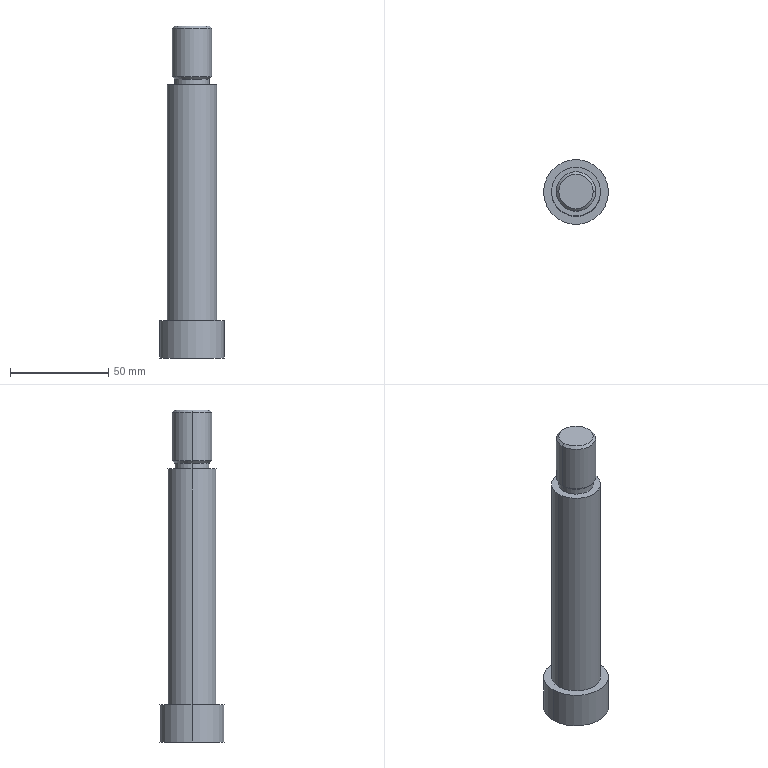Part | Creo | 1 solid | 23 faces | box 33 x 33 x 169 mm | volume 81512 mm3 | plane 11 | cylinder 8 | cone 4 | commonest cylinder face diameters 17.5 x2 20 x2 25 x2 33 x2
STEP:
#1=CARTESIAN_POINT('',(-191.5,290.,11.5));
#2=VERTEX_POINT('',#1);
#3=CARTESIAN_POINT('',(-158.5,290.,11.5));
#4=VERTEX_POINT('',#3);
#5=CARTESIAN_POINT('',(-175.,290.,11.5));
#6=DIRECTION('',(0.,0.,-1.));
#7=DIRECTION('',(-1.,0.,0.));
#8=AXIS2_PLACEMENT_3D('',#5,#6,#7);
#9=CIRCLE('',#8,16.5);
#10=EDGE_CURVE('',#2,#4,#9,.T.);
#11=ORIENTED_EDGE('',*,*,#10,.F.);
#12=CARTESIAN_POINT('',(-175.,290.,11.5));
#13=DIRECTION('',(0.,0.,-1.));
#14=DIRECTION('',(1.,0.,0.));
#15=AXIS2_PLACEMENT_3D('',#12,#13,#14);
#16=CIRCLE('',#15,16.5);
#17=EDGE_CURVE('',#4,#2,#16,.T.);
#18=ORIENTED_EDGE('',*,*,#17,.F.);
#19=EDGE_LOOP('',(#11,#18));
#20=FACE_OUTER_BOUND('',#19,.F.);
#21=CARTESIAN_POINT('',(-166.5,294.907,11.5));
#22=VERTEX_POINT('',#21);
#23=CARTESIAN_POINT('',(-175.,299.815,11.5));
#24=VERTEX_POINT('',#23);
#25=CARTESIAN_POINT('',(-166.5,294.907,11.5));
#26=DIRECTION('',(-0.866,0.5,0.));
#27=VECTOR('',#26,9.815);
#28=LINE('',#25,#27);
#29=EDGE_CURVE('',#22,#24,#28,.T.);
#30=ORIENTED_EDGE('',*,*,#29,.F.);
#31=CARTESIAN_POINT('',(-166.5,285.093,11.5));
#32=VERTEX_POINT('',#31);
#33=CARTESIAN_POINT('',(-166.5,285.093,11.5));
#34=DIRECTION('',(0.,1.,0.));
#35=VECTOR('',#34,9.815);
#36=LINE('',#33,#35);
#37=EDGE_CURVE('',#32,#22,#36,.T.);
#38=ORIENTED_EDGE('',*,*,#37,.F.);
#39=CARTESIAN_POINT('',(-175.,280.185,11.5));
#40=VERTEX_POINT('',#39);
#41=CARTESIAN_POINT('',(-175.,280.185,11.5));
#42=DIRECTION('',(0.866,0.5,0.));
#43=VECTOR('',#42,9.815);
#44=LINE('',#41,#43);
#45=EDGE_CURVE('',#40,#32,#44,.T.);
#46=ORIENTED_EDGE('',*,*,#45,.F.);
#47=CARTESIAN_POINT('',(-183.5,285.093,11.5));
#48=VERTEX_POINT('',#47);
#49=CARTESIAN_POINT('',(-183.5,285.093,11.5));
#50=DIRECTION('',(0.866,-0.5,0.));
#51=VECTOR('',#50,9.815);
#52=LINE('',#49,#51);
#53=EDGE_CURVE('',#48,#40,#52,.T.);
#54=ORIENTED_EDGE('',*,*,#53,.F.);
#55=CARTESIAN_POINT('',(-183.5,294.907,11.5));
#56=VERTEX_POINT('',#55);
#57=CARTESIAN_POINT('',(-183.5,285.093,11.5));
#58=DIRECTION('',(0.,1.,0.));
#59=VECTOR('',#58,9.815);
#60=LINE('',#57,#59);
#61=EDGE_CURVE('',#48,#56,#60,.T.);
#62=ORIENTED_EDGE('',*,*,#61,.T.);
#63=CARTESIAN_POINT('',(-175.,299.815,11.5));
#64=DIRECTION('',(-0.866,-0.5,0.));
#65=VECTOR('',#64,9.815);
#66=LINE('',#63,#65);
#67=EDGE_CURVE('',#24,#56,#66,.T.);
#68=ORIENTED_EDGE('',*,*,#67,.F.);
#69=EDGE_LOOP('',(#30,#38,#46,#54,#62,#68));
#70=FACE_BOUND('',#69,.F.);
#71=CARTESIAN_POINT('',(-175.,290.,11.5));
#72=DIRECTION('',(0.,0.,-1.));
#73=DIRECTION('',(-1.,0.,0.));
#74=AXIS2_PLACEMENT_3D('',#71,#72,#73);
#75=PLANE('',#74);
#76=ADVANCED_FACE('',(#20,#70),#75,.T.);
#77=ORIENTED_EDGE('',*,*,#29,.T.);
#78=CARTESIAN_POINT('',(-175.,299.815,22.5));
#79=VERTEX_POINT('',#78);
#80=CARTESIAN_POINT('',(-175.,299.815,11.5));
#81=DIRECTION('',(0.,0.,1.));
#82=VECTOR('',#81,11.);
#83=LINE('',#80,#82);
#84=EDGE_CURVE('',#24,#79,#83,.T.);
#85=ORIENTED_EDGE('',*,*,#84,.T.);
#86=CARTESIAN_POINT('',(-166.5,294.907,22.5));
#87=VERTEX_POINT('',#86);
#88=CARTESIAN_POINT('',(-175.,299.815,22.5));
#89=DIRECTION('',(0.866,-0.5,0.));
#90=VECTOR('',#89,9.815);
#91=LINE('',#88,#90);
#92=EDGE_CURVE('',#79,#87,#91,.T.);
#93=ORIENTED_EDGE('',*,*,#92,.T.);
#94=CARTESIAN_POINT('',(-166.5,294.907,22.5));
#95=DIRECTION('',(0.,0.,-1.));
#96=VECTOR('',#95,11.);
#97=LINE('',#94,#96);
#98=EDGE_CURVE('',#87,#22,#97,.T.);
#99=ORIENTED_EDGE('',*,*,#98,.T.);
#100=EDGE_LOOP('',(#77,#85,#93,#99));
#101=FACE_OUTER_BOUND('',#100,.F.);
#102=CARTESIAN_POINT('',(-170.75,297.361,30.5));
#103=DIRECTION('',(0.5,0.866,0.));
#104=DIRECTION('',(-0.866,0.5,0.));
#105=AXIS2_PLACEMENT_3D('',#102,#103,#104);
#106=PLANE('',#105);
#107=ADVANCED_FACE('',(#101),#106,.F.);
#108=ORIENTED_EDGE('',*,*,#67,.T.);
#109=CARTESIAN_POINT('',(-183.5,294.907,22.5));
#110=VERTEX_POINT('',#109);
#111=CARTESIAN_POINT('',(-183.5,294.907,22.5));
#112=DIRECTION('',(0.,0.,-1.));
#113=VECTOR('',#112,11.);
#114=LINE('',#111,#113);
#115=EDGE_CURVE('',#110,#56,#114,.T.);
#116=ORIENTED_EDGE('',*,*,#115,.F.);
#117=CARTESIAN_POINT('',(-183.5,294.907,22.5));
#118=DIRECTION('',(0.866,0.5,0.));
#119=VECTOR('',#118,9.815);
#120=LINE('',#117,#119);
#121=EDGE_CURVE('',#110,#79,#120,.T.);
#122=ORIENTED_EDGE('',*,*,#121,.T.);
#123=ORIENTED_EDGE('',*,*,#84,.F.);
#124=EDGE_LOOP('',(#108,#116,#122,#123));
#125=FACE_OUTER_BOUND('',#124,.F.);
#126=CARTESIAN_POINT('',(-179.25,297.361,30.5));
#127=DIRECTION('',(-0.5,0.866,0.));
#128=DIRECTION('',(-0.866,-0.5,0.));
#129=AXIS2_PLACEMENT_3D('',#126,#127,#128);
#130=PLANE('',#129);
#131=ADVANCED_FACE('',(#125),#130,.F.);
#132=ORIENTED_EDGE('',*,*,#115,.T.);
#133=ORIENTED_EDGE('',*,*,#61,.F.);
#134=CARTESIAN_POINT('',(-183.5,285.093,22.5));
#135=VERTEX_POINT('',#134);
#136=CARTESIAN_POINT('',(-183.5,285.093,22.5));
#137=DIRECTION('',(0.,0.,-1.));
#138=VECTOR('',#137,11.);
#139=LINE('',#136,#138);
#140=EDGE_CURVE('',#135,#48,#139,.T.);
#141=ORIENTED_EDGE('',*,*,#140,.F.);
#142=CARTESIAN_POINT('',(-183.5,294.907,22.5));
#143=DIRECTION('',(0.,-1.,0.));
#144=VECTOR('',#143,9.815);
#145=LINE('',#142,#144);
#146=EDGE_CURVE('',#110,#135,#145,.T.);
#147=ORIENTED_EDGE('',*,*,#146,.F.);
#148=EDGE_LOOP('',(#132,#133,#141,#147));
#149=FACE_OUTER_BOUND('',#148,.F.);
#150=CARTESIAN_POINT('',(-183.5,290.,30.5));
#151=DIRECTION('',(1.,0.,0.));
#152=DIRECTION('',(0.,0.,-1.));
#153=AXIS2_PLACEMENT_3D('',#150,#151,#152);
#154=PLANE('',#153);
#155=ADVANCED_FACE('',(#149),#154,.T.);
#156=ORIENTED_EDGE('',*,*,#140,.T.);
#157=ORIENTED_EDGE('',*,*,#53,.T.);
#158=CARTESIAN_POINT('',(-175.,280.185,22.5));
#159=VERTEX_POINT('',#158);
#160=CARTESIAN_POINT('',(-175.,280.185,11.5));
#161=DIRECTION('',(0.,0.,1.));
#162=VECTOR('',#161,11.);
#163=LINE('',#160,#162);
#164=EDGE_CURVE('',#40,#159,#163,.T.);
#165=ORIENTED_EDGE('',*,*,#164,.T.);
#166=CARTESIAN_POINT('',(-175.,280.185,22.5));
#167=DIRECTION('',(-0.866,0.5,0.));
#168=VECTOR('',#167,9.815);
#169=LINE('',#166,#168);
#170=EDGE_CURVE('',#159,#135,#169,.T.);
#171=ORIENTED_EDGE('',*,*,#170,.T.);
#172=EDGE_LOOP('',(#156,#157,#165,#171));
#173=FACE_OUTER_BOUND('',#172,.F.);
#174=CARTESIAN_POINT('',(-179.25,282.639,30.5));
#175=DIRECTION('',(0.5,0.866,0.));
#176=DIRECTION('',(-0.866,0.5,0.));
#177=AXIS2_PLACEMENT_3D('',#174,#175,#176);
#178=PLANE('',#177);
#179=ADVANCED_FACE('',(#173),#178,.T.);
#180=ORIENTED_EDGE('',*,*,#164,.F.);
#181=ORIENTED_EDGE('',*,*,#45,.T.);
#182=CARTESIAN_POINT('',(-166.5,285.093,22.5));
#183=VERTEX_POINT('',#182);
#184=CARTESIAN_POINT('',(-166.5,285.093,22.5));
#185=DIRECTION('',(0.,0.,-1.));
#186=VECTOR('',#185,11.);
#187=LINE('',#184,#186);
#188=EDGE_CURVE('',#183,#32,#187,.T.);
#189=ORIENTED_EDGE('',*,*,#188,.F.);
#190=CARTESIAN_POINT('',(-166.5,285.093,22.5));
#191=DIRECTION('',(-0.866,-0.5,0.));
#192=VECTOR('',#191,9.815);
#193=LINE('',#190,#192);
#194=EDGE_CURVE('',#183,#159,#193,.T.);
#195=ORIENTED_EDGE('',*,*,#194,.T.);
#196=EDGE_LOOP('',(#180,#181,#189,#195));
#197=FACE_OUTER_BOUND('',#196,.F.);
#198=CARTESIAN_POINT('',(-170.75,282.639,30.5));
#199=DIRECTION('',(-0.5,0.866,0.));
#200=DIRECTION('',(-0.866,-0.5,0.));
#201=AXIS2_PLACEMENT_3D('',#198,#199,#200);
#202=PLANE('',#201);
#203=ADVANCED_FACE('',(#197),#202,.T.);
#204=ORIENTED_EDGE('',*,*,#37,.T.);
#205=ORIENTED_EDGE('',*,*,#98,.F.);
#206=CARTESIAN_POINT('',(-166.5,294.907,22.5));
#207=DIRECTION('',(0.,-1.,0.));
#208=VECTOR('',#207,9.815);
#209=LINE('',#206,#208);
#210=EDGE_CURVE('',#87,#183,#209,.T.);
#211=ORIENTED_EDGE('',*,*,#210,.T.);
#212=ORIENTED_EDGE('',*,*,#188,.T.);
#213=EDGE_LOOP('',(#204,#205,#211,#212));
#214=FACE_OUTER_BOUND('',#213,.F.);
#215=CARTESIAN_POINT('',(-166.5,290.,30.5));
#216=DIRECTION('',(1.,0.,0.));
#217=DIRECTION('',(0.,0.,-1.));
#218=AXIS2_PLACEMENT_3D('',#215,#216,#217);
#219=PLANE('',#218);
#220=ADVANCED_FACE('',(#214),#219,.F.);
#221=ORIENTED_EDGE('',*,*,#170,.F.);
#222=ORIENTED_EDGE('',*,*,#194,.F.);
#223=ORIENTED_EDGE('',*,*,#210,.F.);
#224=ORIENTED_EDGE('',*,*,#92,.F.);
#225=ORIENTED_EDGE('',*,*,#121,.F.);
#226=ORIENTED_EDGE('',*,*,#146,.T.);
#227=EDGE_LOOP('',(#221,#222,#223,#224,#225,#226));
#228=FACE_OUTER_BOUND('',#227,.F.);
#229=CARTESIAN_POINT('',(-175.,290.,22.5));
#230=DIRECTION('',(0.,0.,1.));
#231=DIRECTION('',(1.,0.,0.));
#232=AXIS2_PLACEMENT_3D('',#229,#230,#231);
#233=PLANE('',#232);
#234=ADVANCED_FACE('',(#228),#233,.F.);
#235=ORIENTED_EDGE('',*,*,#10,.T.);
#236=CARTESIAN_POINT('',(-158.5,290.,30.5));
#237=VERTEX_POINT('',#236);
#238=CARTESIAN_POINT('',(-158.5,290.,30.5));
#239=DIRECTION('',(0.,0.,-1.));
#240=VECTOR('',#239,19.);
#241=LINE('',#238,#240);
#242=EDGE_CURVE('',#237,#4,#241,.T.);
#243=ORIENTED_EDGE('',*,*,#242,.F.);
#244=CARTESIAN_POINT('',(-191.5,290.,30.5));
#245=VERTEX_POINT('',#244);
#246=CARTESIAN_POINT('',(-175.,290.,30.5));
#247=DIRECTION('',(0.,0.,1.));
#248=DIRECTION('',(1.,0.,0.));
#249=AXIS2_PLACEMENT_3D('',#246,#247,#248);
#250=CIRCLE('',#249,16.5);
#251=EDGE_CURVE('',#237,#245,#250,.T.);
#252=ORIENTED_EDGE('',*,*,#251,.T.);
#253=CARTESIAN_POINT('',(-191.5,290.,30.5));
#254=DIRECTION('',(0.,0.,-1.));
#255=VECTOR('',#254,19.);
#256=LINE('',#253,#255);
#257=EDGE_CURVE('',#245,#2,#256,.T.);
#258=ORIENTED_EDGE('',*,*,#257,.T.);
#259=EDGE_LOOP('',(#235,#243,#252,#258));
#260=FACE_OUTER_BOUND('',#259,.F.);
#261=CARTESIAN_POINT('',(-175.,290.,30.5));
#262=DIRECTION('',(0.,0.,-1.));
#263=DIRECTION('',(-1.,0.,0.));
#264=AXIS2_PLACEMENT_3D('',#261,#262,#263);
#265=CYLINDRICAL_SURFACE('',#264,16.5);
#266=ADVANCED_FACE('',(#260),#265,.T.);
#267=ORIENTED_EDGE('',*,*,#17,.T.);
#268=ORIENTED_EDGE('',*,*,#257,.F.);
#269=CARTESIAN_POINT('',(-175.,290.,30.5));
#270=DIRECTION('',(0.,0.,1.));
#271=DIRECTION('',(-1.,0.,0.));
#272=AXIS2_PLACEMENT_3D('',#269,#270,#271);
#273=CIRCLE('',#272,16.5);
#274=EDGE_CURVE('',#245,#237,#273,.T.);
#275=ORIENTED_EDGE('',*,*,#274,.T.);
#276=ORIENTED_EDGE('',*,*,#242,.T.);
#277=EDGE_LOOP('',(#267,#268,#275,#276));
#278=FACE_OUTER_BOUND('',#277,.F.);
#279=CARTESIAN_POINT('',(-175.,290.,30.5));
#280=DIRECTION('',(0.,0.,-1.));
#281=DIRECTION('',(-1.,0.,0.));
#282=AXIS2_PLACEMENT_3D('',#279,#280,#281);
#283=CYLINDRICAL_SURFACE('',#282,16.5);
#284=ADVANCED_FACE('',(#278),#283,.T.);
#285=ORIENTED_EDGE('',*,*,#274,.F.);
#286=ORIENTED_EDGE('',*,*,#251,.F.);
#287=EDGE_LOOP('',(#285,#286));
#288=FACE_OUTER_BOUND('',#287,.F.);
#289=CARTESIAN_POINT('',(-162.5,290.,30.5));
#290=VERTEX_POINT('',#289);
#291=CARTESIAN_POINT('',(-187.5,290.,30.5));
#292=VERTEX_POINT('',#291);
#293=CARTESIAN_POINT('',(-175.,290.,30.5));
#294=DIRECTION('',(0.,0.,-1.));
#295=DIRECTION('',(1.,0.,0.));
#296=AXIS2_PLACEMENT_3D('',#293,#294,#295);
#297=CIRCLE('',#296,12.5);
#298=EDGE_CURVE('',#290,#292,#297,.T.);
#299=ORIENTED_EDGE('',*,*,#298,.F.);
#300=CARTESIAN_POINT('',(-175.,290.,30.5));
#301=DIRECTION('',(0.,0.,-1.));
#302=DIRECTION('',(-1.,0.,0.));
#303=AXIS2_PLACEMENT_3D('',#300,#301,#302);
#304=CIRCLE('',#303,12.5);
#305=EDGE_CURVE('',#292,#290,#304,.T.);
#306=ORIENTED_EDGE('',*,*,#305,.F.);
#307=EDGE_LOOP('',(#299,#306));
#308=FACE_BOUND('',#307,.F.);
#309=CARTESIAN_POINT('',(-175.,290.,30.5));
#310=DIRECTION('',(0.,0.,1.));
#311=DIRECTION('',(1.,0.,0.));
#312=AXIS2_PLACEMENT_3D('',#309,#310,#311);
#313=PLANE('',#312);
#314=ADVANCED_FACE('',(#288,#308),#313,.T.);
#315=CARTESIAN_POINT('',(-187.5,290.,150.5));
#316=VERTEX_POINT('',#315);
#317=CARTESIAN_POINT('',(-162.5,290.,150.5));
#318=VERTEX_POINT('',#317);
#319=CARTESIAN_POINT('',(-175.,290.,150.5));
#320=DIRECTION('',(0.,0.,1.));
#321=DIRECTION('',(-1.,0.,0.));
#322=AXIS2_PLACEMENT_3D('',#319,#320,#321);
#323=CIRCLE('',#322,12.5);
#324=EDGE_CURVE('',#316,#318,#323,.T.);
#325=ORIENTED_EDGE('',*,*,#324,.T.);
#326=CARTESIAN_POINT('',(-162.5,290.,30.5));
#327=DIRECTION('',(0.,0.,1.));
#328=VECTOR('',#327,120.);
#329=LINE('',#326,#328);
#330=EDGE_CURVE('',#290,#318,#329,.T.);
#331=ORIENTED_EDGE('',*,*,#330,.F.);
#332=ORIENTED_EDGE('',*,*,#298,.T.);
#333=CARTESIAN_POINT('',(-187.5,290.,30.5));
#334=DIRECTION('',(0.,0.,1.));
#335=VECTOR('',#334,120.);
#336=LINE('',#333,#335);
#337=EDGE_CURVE('',#292,#316,#336,.T.);
#338=ORIENTED_EDGE('',*,*,#337,.T.);
#339=EDGE_LOOP('',(#325,#331,#332,#338));
#340=FACE_OUTER_BOUND('',#339,.F.);
#341=CARTESIAN_POINT('',(-175.,290.,100.5));
#342=DIRECTION('',(0.,0.,1.));
#343=DIRECTION('',(1.,0.,0.));
#344=AXIS2_PLACEMENT_3D('',#341,#342,#343);
#345=CYLINDRICAL_SURFACE('',#344,12.5);
#346=ADVANCED_FACE('',(#340),#345,.T.);
#347=ORIENTED_EDGE('',*,*,#324,.F.);
#348=CARTESIAN_POINT('',(-175.,290.,150.5));
#349=DIRECTION('',(0.,0.,1.));
#350=DIRECTION('',(1.,0.,0.));
#351=AXIS2_PLACEMENT_3D('',#348,#349,#350);
#352=CIRCLE('',#351,12.5);
#353=EDGE_CURVE('',#318,#316,#352,.T.);
#354=ORIENTED_EDGE('',*,*,#353,.F.);
#355=EDGE_LOOP('',(#347,#354));
#356=FACE_OUTER_BOUND('',#355,.F.);
#357=CARTESIAN_POINT('',(-166.25,290.,150.5));
#358=VERTEX_POINT('',#357);
#359=CARTESIAN_POINT('',(-183.75,290.,150.5));
#360=VERTEX_POINT('',#359);
#361=CARTESIAN_POINT('',(-175.,290.,150.5));
#362=DIRECTION('',(0.,0.,-1.));
#363=DIRECTION('',(1.,0.,0.));
#364=AXIS2_PLACEMENT_3D('',#361,#362,#363);
#365=CIRCLE('',#364,8.75);
#366=EDGE_CURVE('',#358,#360,#365,.T.);
#367=ORIENTED_EDGE('',*,*,#366,.F.);
#368=CARTESIAN_POINT('',(-175.,290.,150.5));
#369=DIRECTION('',(0.,0.,-1.));
#370=DIRECTION('',(-1.,0.,0.));
#371=AXIS2_PLACEMENT_3D('',#368,#369,#370);
#372=CIRCLE('',#371,8.75);
#373=EDGE_CURVE('',#360,#358,#372,.T.);
#374=ORIENTED_EDGE('',*,*,#373,.F.);
#375=EDGE_LOOP('',(#367,#374));
#376=FACE_BOUND('',#375,.F.);
#377=CARTESIAN_POINT('',(-175.,290.,150.5));
#378=DIRECTION('',(0.,0.,1.));
#379=DIRECTION('',(1.,0.,0.));
#380=AXIS2_PLACEMENT_3D('',#377,#378,#379);
#381=PLANE('',#380);
#382=ADVANCED_FACE('',(#356,#376),#381,.T.);
#383=ORIENTED_EDGE('',*,*,#353,.T.);
#384=ORIENTED_EDGE('',*,*,#337,.F.);
#385=ORIENTED_EDGE('',*,*,#305,.T.);
#386=ORIENTED_EDGE('',*,*,#330,.T.);
#387=EDGE_LOOP('',(#383,#384,#385,#386));
#388=FACE_OUTER_BOUND('',#387,.F.);
#389=CARTESIAN_POINT('',(-175.,290.,100.5));
#390=DIRECTION('',(0.,0.,1.));
#391=DIRECTION('',(1.,0.,0.));
#392=AXIS2_PLACEMENT_3D('',#389,#390,#391);
#393=CYLINDRICAL_SURFACE('',#392,12.5);
#394=ADVANCED_FACE('',(#388),#393,.T.);
#395=CARTESIAN_POINT('',(-183.75,290.,153.5));
#396=VERTEX_POINT('',#395);
#397=CARTESIAN_POINT('',(-166.25,290.,153.5));
#398=VERTEX_POINT('',#397);
#399=CARTESIAN_POINT('',(-175.,290.,153.5));
#400=DIRECTION('',(0.,0.,1.));
#401=DIRECTION('',(-1.,0.,0.));
#402=AXIS2_PLACEMENT_3D('',#399,#400,#401);
#403=CIRCLE('',#402,8.75);
#404=EDGE_CURVE('',#396,#398,#403,.T.);
#405=ORIENTED_EDGE('',*,*,#404,.T.);
#406=CARTESIAN_POINT('',(-166.25,290.,150.5));
#407=DIRECTION('',(0.,0.,1.));
#408=VECTOR('',#407,3.);
#409=LINE('',#406,#408);
#410=EDGE_CURVE('',#358,#398,#409,.T.);
#411=ORIENTED_EDGE('',*,*,#410,.F.);
#412=ORIENTED_EDGE('',*,*,#366,.T.);
#413=CARTESIAN_POINT('',(-183.75,290.,150.5));
#414=DIRECTION('',(0.,0.,1.));
#415=VECTOR('',#414,3.);
#416=LINE('',#413,#415);
#417=EDGE_CURVE('',#360,#396,#416,.T.);
#418=ORIENTED_EDGE('',*,*,#417,.T.);
#419=EDGE_LOOP('',(#405,#411,#412,#418));
#420=FACE_OUTER_BOUND('',#419,.F.);
#421=CARTESIAN_POINT('',(-175.,290.,150.5));
#422=DIRECTION('',(0.,0.,1.));
#423=DIRECTION('',(1.,0.,0.));
#424=AXIS2_PLACEMENT_3D('',#421,#422,#423);
#425=CYLINDRICAL_SURFACE('',#424,8.75);
#426=ADVANCED_FACE('',(#420),#425,.T.);
#427=CARTESIAN_POINT('',(-165.,290.,154.75));
#428=VERTEX_POINT('',#427);
#429=CARTESIAN_POINT('',(-185.,290.,154.75));
#430=VERTEX_POINT('',#429);
#431=CARTESIAN_POINT('',(-175.,290.,154.75));
#432=DIRECTION('',(0.,0.,-1.));
#433=DIRECTION('',(1.,0.,0.));
#434=AXIS2_PLACEMENT_3D('',#431,#432,#433);
#435=CIRCLE('',#434,10.);
#436=EDGE_CURVE('',#428,#430,#435,.T.);
#437=ORIENTED_EDGE('',*,*,#436,.F.);
#438=CARTESIAN_POINT('',(-166.25,290.,153.5));
#439=DIRECTION('',(0.7071,0.,0.7071));
#440=VECTOR('',#439,1.768);
#441=LINE('',#438,#440);
#442=EDGE_CURVE('',#398,#428,#441,.T.);
#443=ORIENTED_EDGE('',*,*,#442,.F.);
#444=ORIENTED_EDGE('',*,*,#404,.F.);
#445=CARTESIAN_POINT('',(-183.75,290.,153.5));
#446=DIRECTION('',(-0.7071,0.,0.7071));
#447=VECTOR('',#446,1.768);
#448=LINE('',#445,#447);
#449=EDGE_CURVE('',#396,#430,#448,.T.);
#450=ORIENTED_EDGE('',*,*,#449,.T.);
#451=EDGE_LOOP('',(#437,#443,#444,#450));
#452=FACE_OUTER_BOUND('',#451,.F.);
#453=CARTESIAN_POINT('',(-175.,290.,154.125));
#454=DIRECTION('',(0.,0.,1.));
#455=DIRECTION('',(1.,0.,0.));
#456=AXIS2_PLACEMENT_3D('',#453,#454,#455);
#457=CONICAL_SURFACE('',#456,9.375,45.);
#458=ADVANCED_FACE('',(#452),#457,.T.);
#459=CARTESIAN_POINT('',(-185.,290.,179.25));
#460=VERTEX_POINT('',#459);
#461=CARTESIAN_POINT('',(-165.,290.,179.25));
#462=VERTEX_POINT('',#461);
#463=CARTESIAN_POINT('',(-175.,290.,179.25));
#464=DIRECTION('',(0.,0.,1.));
#465=DIRECTION('',(-1.,0.,0.));
#466=AXIS2_PLACEMENT_3D('',#463,#464,#465);
#467=CIRCLE('',#466,10.);
#468=EDGE_CURVE('',#460,#462,#467,.T.);
#469=ORIENTED_EDGE('',*,*,#468,.T.);
#470=CARTESIAN_POINT('',(-165.,290.,154.75));
#471=DIRECTION('',(0.,0.,1.));
#472=VECTOR('',#471,24.5);
#473=LINE('',#470,#472);
#474=EDGE_CURVE('',#428,#462,#473,.T.);
#475=ORIENTED_EDGE('',*,*,#474,.F.);
#476=ORIENTED_EDGE('',*,*,#436,.T.);
#477=CARTESIAN_POINT('',(-185.,290.,154.75));
#478=DIRECTION('',(0.,0.,1.));
#479=VECTOR('',#478,24.5);
#480=LINE('',#477,#479);
#481=EDGE_CURVE('',#430,#460,#480,.T.);
#482=ORIENTED_EDGE('',*,*,#481,.T.);
#483=EDGE_LOOP('',(#469,#475,#476,#482));
#484=FACE_OUTER_BOUND('',#483,.F.);
#485=CARTESIAN_POINT('',(-175.,290.,150.5));
#486=DIRECTION('',(0.,0.,1.));
#487=DIRECTION('',(1.,0.,0.));
#488=AXIS2_PLACEMENT_3D('',#485,#486,#487);
#489=CYLINDRICAL_SURFACE('',#488,10.);
#490=ADVANCED_FACE('',(#484),#489,.T.);
#491=CARTESIAN_POINT('',(-183.75,290.,180.5));
#492=VERTEX_POINT('',#491);
#493=CARTESIAN_POINT('',(-166.25,290.,180.5));
#494=VERTEX_POINT('',#493);
#495=CARTESIAN_POINT('',(-175.,290.,180.5));
#496=DIRECTION('',(0.,0.,1.));
#497=DIRECTION('',(-1.,0.,0.));
#498=AXIS2_PLACEMENT_3D('',#495,#496,#497);
#499=CIRCLE('',#498,8.75);
#500=EDGE_CURVE('',#492,#494,#499,.T.);
#501=ORIENTED_EDGE('',*,*,#500,.T.);
#502=CARTESIAN_POINT('',(-166.25,290.,180.5));
#503=DIRECTION('',(0.7071,0.,-0.7071));
#504=VECTOR('',#503,1.768);
#505=LINE('',#502,#504);
#506=EDGE_CURVE('',#494,#462,#505,.T.);
#507=ORIENTED_EDGE('',*,*,#506,.T.);
#508=ORIENTED_EDGE('',*,*,#468,.F.);
#509=CARTESIAN_POINT('',(-183.75,290.,180.5));
#510=DIRECTION('',(-0.7071,0.,-0.7071));
#511=VECTOR('',#510,1.768);
#512=LINE('',#509,#511);
#513=EDGE_CURVE('',#492,#460,#512,.T.);
#514=ORIENTED_EDGE('',*,*,#513,.F.);
#515=EDGE_LOOP('',(#501,#507,#508,#514));
#516=FACE_OUTER_BOUND('',#515,.F.);
#517=CARTESIAN_POINT('',(-175.,290.,179.875));
#518=DIRECTION('',(0.,0.,-1.));
#519=DIRECTION('',(-1.,0.,0.));
#520=AXIS2_PLACEMENT_3D('',#517,#518,#519);
#521=CONICAL_SURFACE('',#520,9.375,45.);
#522=ADVANCED_FACE('',(#516),#521,.T.);
#523=CARTESIAN_POINT('',(-175.,290.,180.5));
#524=DIRECTION('',(0.,0.,1.));
#525=DIRECTION('',(1.,0.,0.));
#526=AXIS2_PLACEMENT_3D('',#523,#524,#525);
#527=CIRCLE('',#526,8.75);
#528=EDGE_CURVE('',#494,#492,#527,.T.);
#529=ORIENTED_EDGE('',*,*,#528,.F.);
#530=ORIENTED_EDGE('',*,*,#500,.F.);
#531=EDGE_LOOP('',(#529,#530));
#532=FACE_OUTER_BOUND('',#531,.F.);
#533=CARTESIAN_POINT('',(-175.,290.,180.5));
#534=DIRECTION('',(0.,0.,1.));
#535=DIRECTION('',(1.,0.,0.));
#536=AXIS2_PLACEMENT_3D('',#533,#534,#535);
#537=PLANE('',#536);
#538=ADVANCED_FACE('',(#532),#537,.T.);
#539=ORIENTED_EDGE('',*,*,#528,.T.);
#540=ORIENTED_EDGE('',*,*,#513,.T.);
#541=CARTESIAN_POINT('',(-175.,290.,179.25));
#542=DIRECTION('',(0.,0.,1.));
#543=DIRECTION('',(1.,0.,0.));
#544=AXIS2_PLACEMENT_3D('',#541,#542,#543);
#545=CIRCLE('',#544,10.);
#546=EDGE_CURVE('',#462,#460,#545,.T.);
#547=ORIENTED_EDGE('',*,*,#546,.F.);
#548=ORIENTED_EDGE('',*,*,#506,.F.);
#549=EDGE_LOOP('',(#539,#540,#547,#548));
#550=FACE_OUTER_BOUND('',#549,.F.);
#551=CARTESIAN_POINT('',(-175.,290.,179.875));
#552=DIRECTION('',(0.,0.,-1.));
#553=DIRECTION('',(-1.,0.,0.));
#554=AXIS2_PLACEMENT_3D('',#551,#552,#553);
#555=CONICAL_SURFACE('',#554,9.375,45.);
#556=ADVANCED_FACE('',(#550),#555,.T.);
#557=ORIENTED_EDGE('',*,*,#546,.T.);
#558=ORIENTED_EDGE('',*,*,#481,.F.);
#559=CARTESIAN_POINT('',(-175.,290.,154.75));
#560=DIRECTION('',(0.,0.,-1.));
#561=DIRECTION('',(-1.,0.,0.));
#562=AXIS2_PLACEMENT_3D('',#559,#560,#561);
#563=CIRCLE('',#562,10.);
#564=EDGE_CURVE('',#430,#428,#563,.T.);
#565=ORIENTED_EDGE('',*,*,#564,.T.);
#566=ORIENTED_EDGE('',*,*,#474,.T.);
#567=EDGE_LOOP('',(#557,#558,#565,#566));
#568=FACE_OUTER_BOUND('',#567,.F.);
#569=CARTESIAN_POINT('',(-175.,290.,150.5));
#570=DIRECTION('',(0.,0.,1.));
#571=DIRECTION('',(1.,0.,0.));
#572=AXIS2_PLACEMENT_3D('',#569,#570,#571);
#573=CYLINDRICAL_SURFACE('',#572,10.);
#574=ADVANCED_FACE('',(#568),#573,.T.);
#575=ORIENTED_EDGE('',*,*,#564,.F.);
#576=ORIENTED_EDGE('',*,*,#449,.F.);
#577=CARTESIAN_POINT('',(-175.,290.,153.5));
#578=DIRECTION('',(0.,0.,1.));
#579=DIRECTION('',(1.,0.,0.));
#580=AXIS2_PLACEMENT_3D('',#577,#578,#579);
#581=CIRCLE('',#580,8.75);
#582=EDGE_CURVE('',#398,#396,#581,.T.);
#583=ORIENTED_EDGE('',*,*,#582,.F.);
#584=ORIENTED_EDGE('',*,*,#442,.T.);
#585=EDGE_LOOP('',(#575,#576,#583,#584));
#586=FACE_OUTER_BOUND('',#585,.F.);
#587=CARTESIAN_POINT('',(-175.,290.,154.125));
#588=DIRECTION('',(0.,0.,1.));
#589=DIRECTION('',(1.,0.,0.));
#590=AXIS2_PLACEMENT_3D('',#587,#588,#589);
#591=CONICAL_SURFACE('',#590,9.375,45.);
#592=ADVANCED_FACE('',(#586),#591,.T.);
#593=ORIENTED_EDGE('',*,*,#582,.T.);
#594=ORIENTED_EDGE('',*,*,#417,.F.);
#595=ORIENTED_EDGE('',*,*,#373,.T.);
#596=ORIENTED_EDGE('',*,*,#410,.T.);
#597=EDGE_LOOP('',(#593,#594,#595,#596));
#598=FACE_OUTER_BOUND('',#597,.F.);
#599=CARTESIAN_POINT('',(-175.,290.,150.5));
#600=DIRECTION('',(0.,0.,1.));
#601=DIRECTION('',(1.,0.,0.));
#602=AXIS2_PLACEMENT_3D('',#599,#600,#601);
#603=CYLINDRICAL_SURFACE('',#602,8.75);
#604=ADVANCED_FACE('',(#598),#603,.T.);
#605=CLOSED_SHELL('',(#76,#107,#131,#155,#179,#203,#220,#234,#266,#284,#314,#346,#382,#394,#426,#458,#490,#522,#538,#556,#574,#592,#604));
#606=MANIFOLD_SOLID_BREP('',#605);
#607=(LENGTH_UNIT()NAMED_UNIT(*)SI_UNIT(.MILLI.,.METRE.));
#608=UNCERTAINTY_MEASURE_WITH_UNIT(LENGTH_MEASURE(0.01753),#607,'','');
#609=(NAMED_UNIT(*)PLANE_ANGLE_UNIT()SI_UNIT($,.RADIAN.));
#610=PLANE_ANGLE_MEASURE_WITH_UNIT(PLANE_ANGLE_MEASURE(0.01745),#609);
#611=(CONVERSION_BASED_UNIT('DEGREE',#610)NAMED_UNIT(*)PLANE_ANGLE_UNIT());
#612=(NAMED_UNIT(*)SI_UNIT($,.STERADIAN.)SOLID_ANGLE_UNIT());
#613=(GEOMETRIC_REPRESENTATION_CONTEXT(3)GLOBAL_UNCERTAINTY_ASSIGNED_CONTEXT((#608))GLOBAL_UNIT_ASSIGNED_CONTEXT((#607,#611,#612))REPRESENTATION_CONTEXT('',''));
#614=ADVANCED_BREP_SHAPE_REPRESENTATION('',(#606),#613);